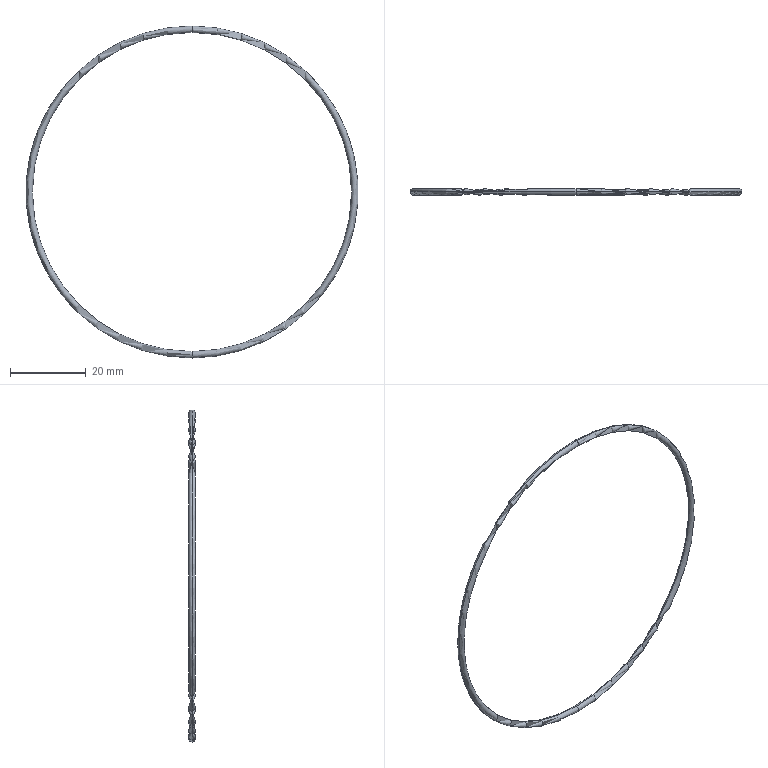Part | SolidWorks | features Revolution 1 | 1 solid | 4 faces | box 87.4 x 1.7 x 87.4 mm | volume 611.109 mm3 | torus 4
STEP:
#1=CARTESIAN_POINT('',(0.,0.,43.7));
#2=VERTEX_POINT('',#1);
#3=CARTESIAN_POINT('',(0.,0.,42.));
#4=VERTEX_POINT('',#3);
#5=CARTESIAN_POINT('',(0.,0.,42.85));
#6=DIRECTION('',(1.,0.,0.));
#7=DIRECTION('',(0.,0.,-1.));
#8=AXIS2_PLACEMENT_3D('',#5,#6,#7);
#9=CIRCLE('',#8,0.85);
#10=EDGE_CURVE('',#2,#4,#9,.T.);
#11=ORIENTED_EDGE('',*,*,#10,.F.);
#12=CARTESIAN_POINT('',(0.,0.,-43.7));
#13=VERTEX_POINT('',#12);
#14=CARTESIAN_POINT('',(0.,0.,0.));
#15=DIRECTION('',(0.,-1.,0.));
#16=DIRECTION('',(0.,0.,-1.));
#17=AXIS2_PLACEMENT_3D('',#14,#15,#16);
#18=CIRCLE('',#17,43.7);
#19=EDGE_CURVE('',#2,#13,#18,.T.);
#20=ORIENTED_EDGE('',*,*,#19,.T.);
#21=CARTESIAN_POINT('',(0.,0.,-42.));
#22=VERTEX_POINT('',#21);
#23=CARTESIAN_POINT('',(0.,0.,-42.85));
#24=DIRECTION('',(-1.,0.,0.));
#25=DIRECTION('',(0.,0.,1.));
#26=AXIS2_PLACEMENT_3D('',#23,#24,#25);
#27=CIRCLE('',#26,0.85);
#28=EDGE_CURVE('',#13,#22,#27,.T.);
#29=ORIENTED_EDGE('',*,*,#28,.T.);
#30=CARTESIAN_POINT('',(0.,0.,0.));
#31=DIRECTION('',(0.,-1.,0.));
#32=DIRECTION('',(0.,0.,-1.));
#33=AXIS2_PLACEMENT_3D('',#30,#31,#32);
#34=CIRCLE('',#33,42.);
#35=EDGE_CURVE('',#4,#22,#34,.T.);
#36=ORIENTED_EDGE('',*,*,#35,.F.);
#37=EDGE_LOOP('',(#11,#20,#29,#36));
#38=FACE_OUTER_BOUND('',#37,.T.);
#39=CARTESIAN_POINT('',(0.,0.,0.));
#40=DIRECTION('',(0.,-1.,0.));
#41=DIRECTION('',(0.,0.,-1.));
#42=AXIS2_PLACEMENT_3D('',#39,#40,#41);
#43=TOROIDAL_SURFACE('',#42,42.85,0.85);
#44=ADVANCED_FACE('',(#38),#43,.T.);
#45=ORIENTED_EDGE('',*,*,#28,.F.);
#46=CARTESIAN_POINT('',(0.,0.,0.));
#47=DIRECTION('',(0.,-1.,0.));
#48=DIRECTION('',(0.,0.,-1.));
#49=AXIS2_PLACEMENT_3D('',#46,#47,#48);
#50=CIRCLE('',#49,43.7);
#51=EDGE_CURVE('',#13,#2,#50,.T.);
#52=ORIENTED_EDGE('',*,*,#51,.T.);
#53=ORIENTED_EDGE('',*,*,#10,.T.);
#54=CARTESIAN_POINT('',(0.,0.,0.));
#55=DIRECTION('',(0.,-1.,0.));
#56=DIRECTION('',(0.,0.,-1.));
#57=AXIS2_PLACEMENT_3D('',#54,#55,#56);
#58=CIRCLE('',#57,42.);
#59=EDGE_CURVE('',#22,#4,#58,.T.);
#60=ORIENTED_EDGE('',*,*,#59,.F.);
#61=EDGE_LOOP('',(#45,#52,#53,#60));
#62=FACE_OUTER_BOUND('',#61,.T.);
#63=CARTESIAN_POINT('',(0.,0.,0.));
#64=DIRECTION('',(0.,-1.,0.));
#65=DIRECTION('',(0.,0.,-1.));
#66=AXIS2_PLACEMENT_3D('',#63,#64,#65);
#67=TOROIDAL_SURFACE('',#66,42.85,0.85);
#68=ADVANCED_FACE('',(#62),#67,.T.);
#69=ORIENTED_EDGE('',*,*,#51,.F.);
#70=CARTESIAN_POINT('',(0.,0.,-42.85));
#71=DIRECTION('',(-1.,0.,0.));
#72=DIRECTION('',(0.,0.,1.));
#73=AXIS2_PLACEMENT_3D('',#70,#71,#72);
#74=CIRCLE('',#73,0.85);
#75=EDGE_CURVE('',#22,#13,#74,.T.);
#76=ORIENTED_EDGE('',*,*,#75,.F.);
#77=ORIENTED_EDGE('',*,*,#59,.T.);
#78=CARTESIAN_POINT('',(0.,0.,42.85));
#79=DIRECTION('',(1.,0.,0.));
#80=DIRECTION('',(0.,0.,-1.));
#81=AXIS2_PLACEMENT_3D('',#78,#79,#80);
#82=CIRCLE('',#81,0.85);
#83=EDGE_CURVE('',#4,#2,#82,.T.);
#84=ORIENTED_EDGE('',*,*,#83,.T.);
#85=EDGE_LOOP('',(#69,#76,#77,#84));
#86=FACE_OUTER_BOUND('',#85,.T.);
#87=CARTESIAN_POINT('',(0.,0.,0.));
#88=DIRECTION('',(0.,-1.,0.));
#89=DIRECTION('',(0.,0.,-1.));
#90=AXIS2_PLACEMENT_3D('',#87,#88,#89);
#91=TOROIDAL_SURFACE('',#90,42.85,0.85);
#92=ADVANCED_FACE('',(#86),#91,.T.);
#93=ORIENTED_EDGE('',*,*,#19,.F.);
#94=ORIENTED_EDGE('',*,*,#83,.F.);
#95=ORIENTED_EDGE('',*,*,#35,.T.);
#96=ORIENTED_EDGE('',*,*,#75,.T.);
#97=EDGE_LOOP('',(#93,#94,#95,#96));
#98=FACE_OUTER_BOUND('',#97,.T.);
#99=CARTESIAN_POINT('',(0.,0.,0.));
#100=DIRECTION('',(0.,-1.,0.));
#101=DIRECTION('',(0.,0.,-1.));
#102=AXIS2_PLACEMENT_3D('',#99,#100,#101);
#103=TOROIDAL_SURFACE('',#102,42.85,0.85);
#104=ADVANCED_FACE('',(#98),#103,.T.);
#105=CLOSED_SHELL('',(#44,#68,#92,#104));
#106=MANIFOLD_SOLID_BREP('',#105);
#107=CARTESIAN_POINT('',(0.,0.,0.));
#108=DIRECTION('',(0.,0.,1.));
#109=DIRECTION('',(1.,0.,0.));
#110=AXIS2_PLACEMENT_3D('',#107,#108,#109);
#111=(LENGTH_UNIT()NAMED_UNIT(*)SI_UNIT(.MILLI.,.METRE.));
#112=UNCERTAINTY_MEASURE_WITH_UNIT(LENGTH_MEASURE(0.00001),#111,'','');
#113=(NAMED_UNIT(*)PLANE_ANGLE_UNIT()SI_UNIT($,.RADIAN.));
#114=(NAMED_UNIT(*)SI_UNIT($,.STERADIAN.)SOLID_ANGLE_UNIT());
#115=(GEOMETRIC_REPRESENTATION_CONTEXT(3)GLOBAL_UNCERTAINTY_ASSIGNED_CONTEXT((#112))GLOBAL_UNIT_ASSIGNED_CONTEXT((#111,#113,#114))REPRESENTATION_CONTEXT('',''));
#116=ADVANCED_BREP_SHAPE_REPRESENTATION('',(#106,#110),#115);